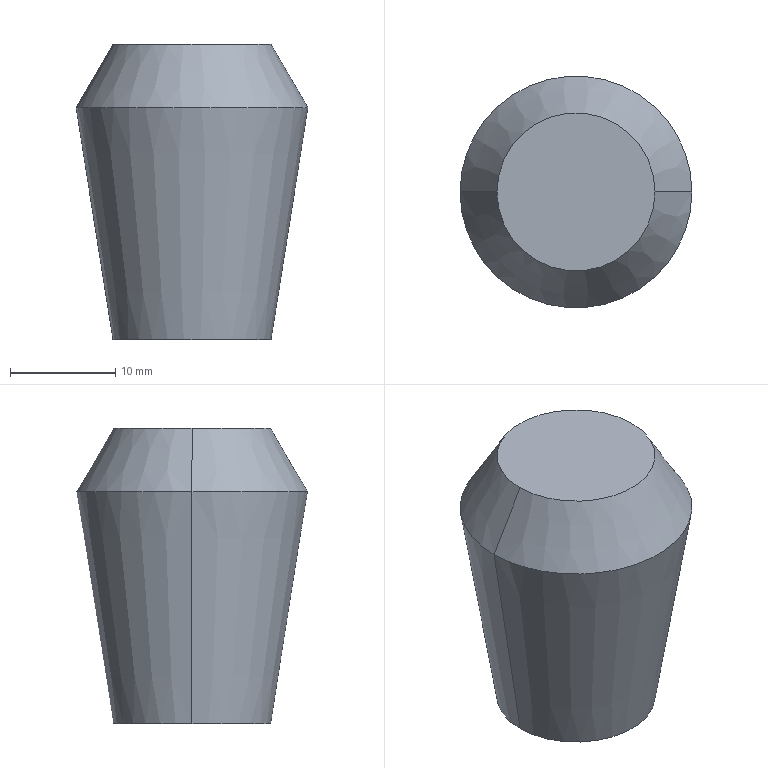Part | SolidWorks | features HoleWzd 1, Revolution 1 | 1 solid | 10 faces | box 22 x 22 x 28 mm | volume 7214 mm3 | cone 6 | cylinder 2 | plane 2 | commonest cylinder face diameters 5 x2
STEP:
#1=CARTESIAN_POINT('',(2.5,0.,-8.));
#2=VERTEX_POINT('',#1);
#3=CARTESIAN_POINT('',(-2.5,0.,-8.));
#4=VERTEX_POINT('',#3);
#5=CARTESIAN_POINT('',(0.,0.,-8.));
#6=DIRECTION('',(0.,0.,-1.));
#7=DIRECTION('',(-1.,0.,0.));
#8=AXIS2_PLACEMENT_3D('',#5,#6,#7);
#9=CIRCLE('',#8,2.5);
#10=EDGE_CURVE('',#2,#4,#9,.T.);
#11=ORIENTED_EDGE('',*,*,#10,.F.);
#12=CARTESIAN_POINT('',(2.5,0.,-28.));
#13=VERTEX_POINT('',#12);
#14=CARTESIAN_POINT('',(2.5,0.,-28.));
#15=DIRECTION('',(0.,0.,-1.));
#16=VECTOR('',#15,1000.);
#17=LINE('',#14,#16);
#18=EDGE_CURVE('',#2,#13,#17,.T.);
#19=ORIENTED_EDGE('',*,*,#18,.T.);
#20=CARTESIAN_POINT('',(-2.5,0.,-28.));
#21=VERTEX_POINT('',#20);
#22=CARTESIAN_POINT('',(0.,0.,-28.));
#23=DIRECTION('',(0.,0.,-1.));
#24=DIRECTION('',(-1.,0.,0.));
#25=AXIS2_PLACEMENT_3D('',#22,#23,#24);
#26=CIRCLE('',#25,2.5);
#27=EDGE_CURVE('',#13,#21,#26,.T.);
#28=ORIENTED_EDGE('',*,*,#27,.T.);
#29=CARTESIAN_POINT('',(-2.5,0.,-28.));
#30=DIRECTION('',(0.,0.,-1.));
#31=VECTOR('',#30,1000.);
#32=LINE('',#29,#31);
#33=EDGE_CURVE('',#4,#21,#32,.T.);
#34=ORIENTED_EDGE('',*,*,#33,.F.);
#35=EDGE_LOOP('',(#11,#19,#28,#34));
#36=FACE_OUTER_BOUND('',#35,.T.);
#37=CARTESIAN_POINT('',(0.,0.,-28.));
#38=DIRECTION('',(0.,0.,-1.));
#39=DIRECTION('',(-1.,0.,0.));
#40=AXIS2_PLACEMENT_3D('',#37,#38,#39);
#41=CYLINDRICAL_SURFACE('',#40,2.5);
#42=ADVANCED_FACE('',(#36),#41,.F.);
#43=CARTESIAN_POINT('',(0.,0.,-6.498));
#44=VERTEX_POINT('',#43);
#45=CARTESIAN_POINT('',(-2.5,0.,-8.));
#46=DIRECTION('',(-0.8572,0.,-0.515));
#47=VECTOR('',#46,1000.);
#48=LINE('',#45,#47);
#49=EDGE_CURVE('',#44,#4,#48,.T.);
#50=ORIENTED_EDGE('',*,*,#49,.F.);
#51=CARTESIAN_POINT('',(2.5,0.,-8.));
#52=DIRECTION('',(0.8572,0.,-0.515));
#53=VECTOR('',#52,1000.);
#54=LINE('',#51,#53);
#55=EDGE_CURVE('',#44,#2,#54,.T.);
#56=ORIENTED_EDGE('',*,*,#55,.T.);
#57=ORIENTED_EDGE('',*,*,#10,.T.);
#58=EDGE_LOOP('',(#50,#56,#57));
#59=FACE_OUTER_BOUND('',#58,.T.);
#60=CARTESIAN_POINT('',(0.,0.,-8.));
#61=DIRECTION('',(0.,0.,-1.));
#62=DIRECTION('',(-1.,0.,0.));
#63=AXIS2_PLACEMENT_3D('',#60,#61,#62);
#64=CONICAL_SURFACE('',#63,2.5,1.03);
#65=ADVANCED_FACE('',(#59),#64,.F.);
#66=CARTESIAN_POINT('',(7.5,0.,-28.));
#67=VERTEX_POINT('',#66);
#68=CARTESIAN_POINT('',(-7.5,0.,-28.));
#69=VERTEX_POINT('',#68);
#70=CARTESIAN_POINT('',(0.,0.,-28.));
#71=DIRECTION('',(0.,0.,1.));
#72=DIRECTION('',(1.,0.,0.));
#73=AXIS2_PLACEMENT_3D('',#70,#71,#72);
#74=CIRCLE('',#73,7.5);
#75=EDGE_CURVE('',#67,#69,#74,.T.);
#76=ORIENTED_EDGE('',*,*,#75,.T.);
#77=CARTESIAN_POINT('',(-11.,0.,-6.));
#78=VERTEX_POINT('',#77);
#79=CARTESIAN_POINT('',(-7.5,0.,-28.));
#80=DIRECTION('',(-0.1571,0.,0.9876));
#81=VECTOR('',#80,1000.);
#82=LINE('',#79,#81);
#83=EDGE_CURVE('',#69,#78,#82,.T.);
#84=ORIENTED_EDGE('',*,*,#83,.T.);
#85=CARTESIAN_POINT('',(11.,0.,-6.));
#86=VERTEX_POINT('',#85);
#87=CARTESIAN_POINT('',(0.,0.,-6.));
#88=DIRECTION('',(0.,0.,1.));
#89=DIRECTION('',(1.,0.,0.));
#90=AXIS2_PLACEMENT_3D('',#87,#88,#89);
#91=CIRCLE('',#90,11.);
#92=EDGE_CURVE('',#86,#78,#91,.T.);
#93=ORIENTED_EDGE('',*,*,#92,.F.);
#94=CARTESIAN_POINT('',(7.5,0.,-28.));
#95=DIRECTION('',(0.1571,0.,0.9876));
#96=VECTOR('',#95,1000.);
#97=LINE('',#94,#96);
#98=EDGE_CURVE('',#67,#86,#97,.T.);
#99=ORIENTED_EDGE('',*,*,#98,.F.);
#100=EDGE_LOOP('',(#76,#84,#93,#99));
#101=FACE_OUTER_BOUND('',#100,.T.);
#102=CARTESIAN_POINT('',(0.,0.,-28.));
#103=DIRECTION('',(0.,0.,1.));
#104=DIRECTION('',(1.,0.,0.));
#105=AXIS2_PLACEMENT_3D('',#102,#103,#104);
#106=CONICAL_SURFACE('',#105,7.5,0.1578);
#107=ADVANCED_FACE('',(#101),#106,.T.);
#108=CARTESIAN_POINT('',(7.5,0.,0.));
#109=VERTEX_POINT('',#108);
#110=CARTESIAN_POINT('',(-7.5,0.,0.));
#111=VERTEX_POINT('',#110);
#112=CARTESIAN_POINT('',(0.,0.,0.));
#113=DIRECTION('',(0.,0.,1.));
#114=DIRECTION('',(1.,0.,0.));
#115=AXIS2_PLACEMENT_3D('',#112,#113,#114);
#116=CIRCLE('',#115,7.5);
#117=EDGE_CURVE('',#109,#111,#116,.T.);
#118=ORIENTED_EDGE('',*,*,#117,.F.);
#119=CARTESIAN_POINT('',(11.,0.,-6.));
#120=DIRECTION('',(0.5039,0.,-0.8638));
#121=VECTOR('',#120,1000.);
#122=LINE('',#119,#121);
#123=EDGE_CURVE('',#109,#86,#122,.T.);
#124=ORIENTED_EDGE('',*,*,#123,.T.);
#125=ORIENTED_EDGE('',*,*,#92,.T.);
#126=CARTESIAN_POINT('',(-11.,0.,-6.));
#127=DIRECTION('',(-0.5039,0.,-0.8638));
#128=VECTOR('',#127,1000.);
#129=LINE('',#126,#128);
#130=EDGE_CURVE('',#111,#78,#129,.T.);
#131=ORIENTED_EDGE('',*,*,#130,.F.);
#132=EDGE_LOOP('',(#118,#124,#125,#131));
#133=FACE_OUTER_BOUND('',#132,.T.);
#134=CARTESIAN_POINT('',(0.,0.,-6.));
#135=DIRECTION('',(0.,0.,-1.));
#136=DIRECTION('',(-1.,0.,0.));
#137=AXIS2_PLACEMENT_3D('',#134,#135,#136);
#138=CONICAL_SURFACE('',#137,11.,0.5281);
#139=ADVANCED_FACE('',(#133),#138,.T.);
#140=CARTESIAN_POINT('',(0.,0.,0.));
#141=DIRECTION('',(0.,0.,1.));
#142=DIRECTION('',(1.,0.,0.));
#143=AXIS2_PLACEMENT_3D('',#140,#141,#142);
#144=CIRCLE('',#143,7.5);
#145=EDGE_CURVE('',#111,#109,#144,.T.);
#146=ORIENTED_EDGE('',*,*,#145,.T.);
#147=ORIENTED_EDGE('',*,*,#117,.T.);
#148=EDGE_LOOP('',(#146,#147));
#149=FACE_OUTER_BOUND('',#148,.T.);
#150=CARTESIAN_POINT('',(0.,0.,0.));
#151=DIRECTION('',(0.,0.,-1.));
#152=DIRECTION('',(-1.,0.,0.));
#153=AXIS2_PLACEMENT_3D('',#150,#151,#152);
#154=PLANE('',#153);
#155=ADVANCED_FACE('',(#149),#154,.F.);
#156=ORIENTED_EDGE('',*,*,#123,.F.);
#157=ORIENTED_EDGE('',*,*,#145,.F.);
#158=ORIENTED_EDGE('',*,*,#130,.T.);
#159=CARTESIAN_POINT('',(0.,0.,-6.));
#160=DIRECTION('',(0.,0.,1.));
#161=DIRECTION('',(1.,0.,0.));
#162=AXIS2_PLACEMENT_3D('',#159,#160,#161);
#163=CIRCLE('',#162,11.);
#164=EDGE_CURVE('',#78,#86,#163,.T.);
#165=ORIENTED_EDGE('',*,*,#164,.T.);
#166=EDGE_LOOP('',(#156,#157,#158,#165));
#167=FACE_OUTER_BOUND('',#166,.T.);
#168=CARTESIAN_POINT('',(0.,0.,-6.));
#169=DIRECTION('',(0.,0.,-1.));
#170=DIRECTION('',(-1.,0.,0.));
#171=AXIS2_PLACEMENT_3D('',#168,#169,#170);
#172=CONICAL_SURFACE('',#171,11.,0.5281);
#173=ADVANCED_FACE('',(#167),#172,.T.);
#174=ORIENTED_EDGE('',*,*,#83,.F.);
#175=CARTESIAN_POINT('',(0.,0.,-28.));
#176=DIRECTION('',(0.,0.,1.));
#177=DIRECTION('',(1.,0.,0.));
#178=AXIS2_PLACEMENT_3D('',#175,#176,#177);
#179=CIRCLE('',#178,7.5);
#180=EDGE_CURVE('',#69,#67,#179,.T.);
#181=ORIENTED_EDGE('',*,*,#180,.T.);
#182=ORIENTED_EDGE('',*,*,#98,.T.);
#183=ORIENTED_EDGE('',*,*,#164,.F.);
#184=EDGE_LOOP('',(#174,#181,#182,#183));
#185=FACE_OUTER_BOUND('',#184,.T.);
#186=CARTESIAN_POINT('',(0.,0.,-28.));
#187=DIRECTION('',(0.,0.,1.));
#188=DIRECTION('',(1.,0.,0.));
#189=AXIS2_PLACEMENT_3D('',#186,#187,#188);
#190=CONICAL_SURFACE('',#189,7.5,0.1578);
#191=ADVANCED_FACE('',(#185),#190,.T.);
#192=CARTESIAN_POINT('',(0.,0.,-28.));
#193=DIRECTION('',(0.,0.,-1.));
#194=DIRECTION('',(-1.,0.,0.));
#195=AXIS2_PLACEMENT_3D('',#192,#193,#194);
#196=CIRCLE('',#195,2.5);
#197=EDGE_CURVE('',#21,#13,#196,.T.);
#198=ORIENTED_EDGE('',*,*,#197,.F.);
#199=ORIENTED_EDGE('',*,*,#27,.F.);
#200=EDGE_LOOP('',(#198,#199));
#201=FACE_BOUND('',#200,.T.);
#202=ORIENTED_EDGE('',*,*,#75,.F.);
#203=ORIENTED_EDGE('',*,*,#180,.F.);
#204=EDGE_LOOP('',(#202,#203));
#205=FACE_OUTER_BOUND('',#204,.T.);
#206=CARTESIAN_POINT('',(-7.5,0.,-28.));
#207=DIRECTION('',(0.,0.,1.));
#208=DIRECTION('',(1.,0.,0.));
#209=AXIS2_PLACEMENT_3D('',#206,#207,#208);
#210=PLANE('',#209);
#211=ADVANCED_FACE('',(#201,#205),#210,.F.);
#212=ORIENTED_EDGE('',*,*,#55,.F.);
#213=ORIENTED_EDGE('',*,*,#49,.T.);
#214=CARTESIAN_POINT('',(0.,0.,-8.));
#215=DIRECTION('',(0.,0.,-1.));
#216=DIRECTION('',(-1.,0.,0.));
#217=AXIS2_PLACEMENT_3D('',#214,#215,#216);
#218=CIRCLE('',#217,2.5);
#219=EDGE_CURVE('',#4,#2,#218,.T.);
#220=ORIENTED_EDGE('',*,*,#219,.T.);
#221=EDGE_LOOP('',(#212,#213,#220));
#222=FACE_OUTER_BOUND('',#221,.T.);
#223=CARTESIAN_POINT('',(0.,0.,-8.));
#224=DIRECTION('',(0.,0.,-1.));
#225=DIRECTION('',(-1.,0.,0.));
#226=AXIS2_PLACEMENT_3D('',#223,#224,#225);
#227=CONICAL_SURFACE('',#226,2.5,1.03);
#228=ADVANCED_FACE('',(#222),#227,.F.);
#229=ORIENTED_EDGE('',*,*,#18,.F.);
#230=ORIENTED_EDGE('',*,*,#219,.F.);
#231=ORIENTED_EDGE('',*,*,#33,.T.);
#232=ORIENTED_EDGE('',*,*,#197,.T.);
#233=EDGE_LOOP('',(#229,#230,#231,#232));
#234=FACE_OUTER_BOUND('',#233,.T.);
#235=CARTESIAN_POINT('',(0.,0.,-28.));
#236=DIRECTION('',(0.,0.,-1.));
#237=DIRECTION('',(-1.,0.,0.));
#238=AXIS2_PLACEMENT_3D('',#235,#236,#237);
#239=CYLINDRICAL_SURFACE('',#238,2.5);
#240=ADVANCED_FACE('',(#234),#239,.F.);
#241=CLOSED_SHELL('',(#42,#65,#107,#139,#155,#173,#191,#211,#228,#240));
#242=MANIFOLD_SOLID_BREP('',#241);
#243=CARTESIAN_POINT('',(0.,0.,0.));
#244=DIRECTION('',(0.,0.,1.));
#245=DIRECTION('',(1.,0.,0.));
#246=AXIS2_PLACEMENT_3D('',#243,#244,#245);
#247=(LENGTH_UNIT()NAMED_UNIT(*)SI_UNIT(.MILLI.,.METRE.));
#248=UNCERTAINTY_MEASURE_WITH_UNIT(LENGTH_MEASURE(0.00001),#247,'','');
#249=(NAMED_UNIT(*)PLANE_ANGLE_UNIT()SI_UNIT($,.RADIAN.));
#250=(NAMED_UNIT(*)SI_UNIT($,.STERADIAN.)SOLID_ANGLE_UNIT());
#251=(GEOMETRIC_REPRESENTATION_CONTEXT(3)GLOBAL_UNCERTAINTY_ASSIGNED_CONTEXT((#248))GLOBAL_UNIT_ASSIGNED_CONTEXT((#247,#249,#250))REPRESENTATION_CONTEXT('',''));
#252=ADVANCED_BREP_SHAPE_REPRESENTATION('',(#242,#246),#251);